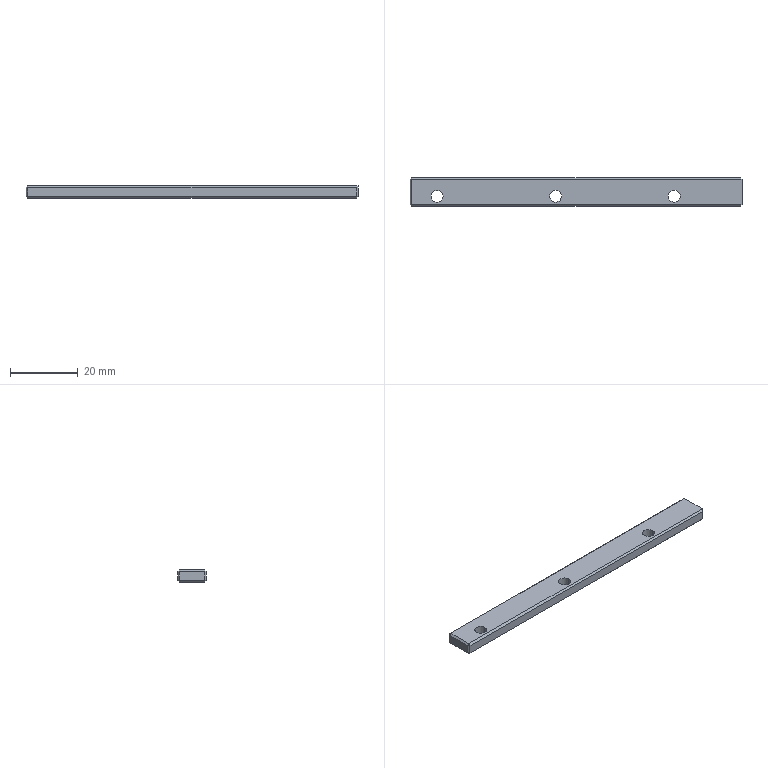Part | STEP file | Harpoon track cover plate_Default | 1 solid | 29 faces | box 98 x 8.5 x 3.6 mm | volume 2841 mm3 | plane 23 | cylinder 6 | commonest cylinder face diameters 3.5 x6